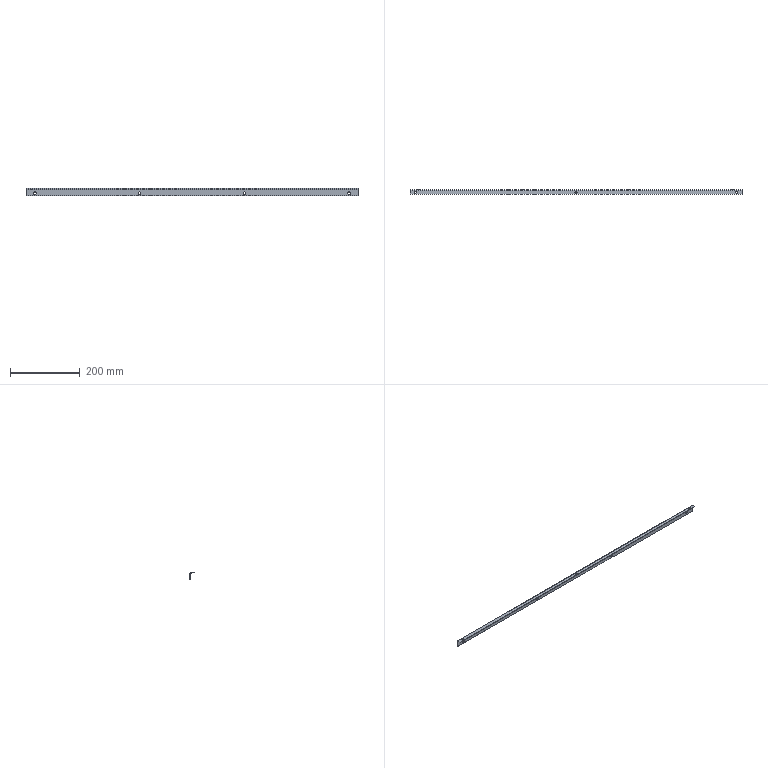Part | NX | features solid 2 | 1 solid | 24 faces | box 950 x 12.085 x 21.546 mm | volume 42798 mm3 | cylinder 16 | plane 8 | commonest cylinder face diameters 8.1 x8 6 x7 3 x1
STEP:
#1=CARTESIAN_POINT('',(626.,-1461.985,109.849));
#2=VERTEX_POINT('',#1);
#3=CARTESIAN_POINT('',(626.,-1462.116,108.354));
#4=VERTEX_POINT('',#3);
#5=CARTESIAN_POINT('',(626.,-1379.29,1055.059));
#6=DIRECTION('',(0.,-0.08716,-0.9962));
#7=VECTOR('',#6,1000.);
#8=LINE('',#5,#7);
#9=EDGE_CURVE('',#2,#4,#8,.T.);
#10=ORIENTED_EDGE('',*,*,#9,.F.);
#11=CARTESIAN_POINT('',(626.,-1467.962,110.372));
#12=VERTEX_POINT('',#11);
#13=CARTESIAN_POINT('',(626.,-1464.973,110.11));
#14=DIRECTION('',(0.,0.08716,0.9962));
#15=DIRECTION('',(0.,0.9962,-0.08716));
#16=AXIS2_PLACEMENT_3D('',#13,#14,#15);
#17=CIRCLE('',#16,3.);
#18=EDGE_CURVE('',#2,#12,#17,.T.);
#19=ORIENTED_EDGE('',*,*,#18,.T.);
#20=CARTESIAN_POINT('',(626.,-1468.093,108.877));
#21=VERTEX_POINT('',#20);
#22=CARTESIAN_POINT('',(626.,-1385.267,1055.582));
#23=DIRECTION('',(0.,-0.08716,-0.9962));
#24=VECTOR('',#23,1000.);
#25=LINE('',#22,#24);
#26=EDGE_CURVE('',#21,#12,#25,.F.);
#27=ORIENTED_EDGE('',*,*,#26,.F.);
#28=CARTESIAN_POINT('',(626.,-1465.104,108.616));
#29=DIRECTION('',(0.,-0.08716,-0.9962));
#30=DIRECTION('',(-1.,0.,0.));
#31=AXIS2_PLACEMENT_3D('',#28,#29,#30);
#32=CIRCLE('',#31,3.);
#33=EDGE_CURVE('',#21,#4,#32,.T.);
#34=ORIENTED_EDGE('',*,*,#33,.T.);
#35=EDGE_LOOP('',(#10,#19,#27,#34));
#36=FACE_BOUND('',#35,.T.);
#37=CARTESIAN_POINT('',(626.,-1382.278,1055.321));
#38=DIRECTION('',(0.,-0.08716,-0.9962));
#39=DIRECTION('',(0.,-0.9962,0.08716));
#40=AXIS2_PLACEMENT_3D('',#37,#38,#39);
#41=CYLINDRICAL_SURFACE('',#40,3.);
#42=ADVANCED_FACE('',(#36),#41,.F.);
#43=CARTESIAN_POINT('',(-294.,-1461.985,109.849));
#44=VERTEX_POINT('',#43);
#45=CARTESIAN_POINT('',(-294.,-1462.116,108.354));
#46=VERTEX_POINT('',#45);
#47=CARTESIAN_POINT('',(-294.,-1379.29,1055.059));
#48=DIRECTION('',(0.,-0.08716,-0.9962));
#49=VECTOR('',#48,1000.);
#50=LINE('',#47,#49);
#51=EDGE_CURVE('',#44,#46,#50,.T.);
#52=ORIENTED_EDGE('',*,*,#51,.F.);
#53=CARTESIAN_POINT('',(-294.,-1467.962,110.372));
#54=VERTEX_POINT('',#53);
#55=CARTESIAN_POINT('',(-294.,-1464.973,110.11));
#56=DIRECTION('',(0.,0.08716,0.9962));
#57=DIRECTION('',(0.,0.9962,-0.08716));
#58=AXIS2_PLACEMENT_3D('',#55,#56,#57);
#59=CIRCLE('',#58,3.);
#60=EDGE_CURVE('',#44,#54,#59,.T.);
#61=ORIENTED_EDGE('',*,*,#60,.T.);
#62=CARTESIAN_POINT('',(-294.,-1468.093,108.877));
#63=VERTEX_POINT('',#62);
#64=CARTESIAN_POINT('',(-294.,-1385.267,1055.582));
#65=DIRECTION('',(0.,-0.08716,-0.9962));
#66=VECTOR('',#65,1000.);
#67=LINE('',#64,#66);
#68=EDGE_CURVE('',#63,#54,#67,.F.);
#69=ORIENTED_EDGE('',*,*,#68,.F.);
#70=CARTESIAN_POINT('',(-294.,-1465.104,108.616));
#71=DIRECTION('',(0.,-0.08716,-0.9962));
#72=DIRECTION('',(-1.,0.,0.));
#73=AXIS2_PLACEMENT_3D('',#70,#71,#72);
#74=CIRCLE('',#73,3.);
#75=EDGE_CURVE('',#63,#46,#74,.T.);
#76=ORIENTED_EDGE('',*,*,#75,.T.);
#77=EDGE_LOOP('',(#52,#61,#69,#76));
#78=FACE_BOUND('',#77,.T.);
#79=CARTESIAN_POINT('',(-294.,-1382.278,1055.321));
#80=DIRECTION('',(0.,-0.08716,-0.9962));
#81=DIRECTION('',(0.,-0.9962,0.08716));
#82=AXIS2_PLACEMENT_3D('',#79,#80,#81);
#83=CYLINDRICAL_SURFACE('',#82,3.);
#84=ADVANCED_FACE('',(#78),#83,.F.);
#85=CARTESIAN_POINT('',(166.,-1461.985,109.849));
#86=VERTEX_POINT('',#85);
#87=CARTESIAN_POINT('',(166.,-1462.116,108.354));
#88=VERTEX_POINT('',#87);
#89=CARTESIAN_POINT('',(166.,-1379.29,1055.059));
#90=DIRECTION('',(0.,-0.08716,-0.9962));
#91=VECTOR('',#90,1000.);
#92=LINE('',#89,#91);
#93=EDGE_CURVE('',#86,#88,#92,.T.);
#94=ORIENTED_EDGE('',*,*,#93,.F.);
#95=CARTESIAN_POINT('',(166.,-1467.962,110.372));
#96=VERTEX_POINT('',#95);
#97=CARTESIAN_POINT('',(166.,-1464.973,110.11));
#98=DIRECTION('',(0.,0.08716,0.9962));
#99=DIRECTION('',(0.,0.9962,-0.08716));
#100=AXIS2_PLACEMENT_3D('',#97,#98,#99);
#101=CIRCLE('',#100,3.);
#102=EDGE_CURVE('',#86,#96,#101,.T.);
#103=ORIENTED_EDGE('',*,*,#102,.T.);
#104=CARTESIAN_POINT('',(166.,-1468.093,108.877));
#105=VERTEX_POINT('',#104);
#106=CARTESIAN_POINT('',(166.,-1385.267,1055.582));
#107=DIRECTION('',(0.,-0.08716,-0.9962));
#108=VECTOR('',#107,1000.);
#109=LINE('',#106,#108);
#110=EDGE_CURVE('',#105,#96,#109,.F.);
#111=ORIENTED_EDGE('',*,*,#110,.F.);
#112=CARTESIAN_POINT('',(166.,-1465.104,108.616));
#113=DIRECTION('',(0.,-0.08716,-0.9962));
#114=DIRECTION('',(-1.,0.,0.));
#115=AXIS2_PLACEMENT_3D('',#112,#113,#114);
#116=CIRCLE('',#115,3.);
#117=EDGE_CURVE('',#105,#88,#116,.T.);
#118=ORIENTED_EDGE('',*,*,#117,.T.);
#119=EDGE_LOOP('',(#94,#103,#111,#118));
#120=FACE_BOUND('',#119,.T.);
#121=CARTESIAN_POINT('',(166.,-1382.278,1055.321));
#122=DIRECTION('',(0.,-0.08716,-0.9962));
#123=DIRECTION('',(0.,-0.9962,0.08716));
#124=AXIS2_PLACEMENT_3D('',#121,#122,#123);
#125=CYLINDRICAL_SURFACE('',#124,3.);
#126=ADVANCED_FACE('',(#120),#125,.F.);
#127=CARTESIAN_POINT('',(-284.,-1459.5,91.95));
#128=VERTEX_POINT('',#127);
#129=CARTESIAN_POINT('',(-284.,-1458.,91.95));
#130=VERTEX_POINT('',#129);
#131=CARTESIAN_POINT('',(-284.,-509.179,91.95));
#132=DIRECTION('',(0.,-1.,0.));
#133=VECTOR('',#132,1000.);
#134=LINE('',#131,#133);
#135=EDGE_CURVE('',#128,#130,#134,.F.);
#136=ORIENTED_EDGE('',*,*,#135,.T.);
#137=CARTESIAN_POINT('',(-284.,-1458.,100.05));
#138=VERTEX_POINT('',#137);
#139=CARTESIAN_POINT('',(-284.,-1458.,96.));
#140=DIRECTION('',(0.,-1.,0.));
#141=DIRECTION('',(0.,0.,-1.));
#142=AXIS2_PLACEMENT_3D('',#139,#140,#141);
#143=CIRCLE('',#142,4.05);
#144=EDGE_CURVE('',#138,#130,#143,.T.);
#145=ORIENTED_EDGE('',*,*,#144,.F.);
#146=CARTESIAN_POINT('',(-284.,-1459.5,100.05));
#147=VERTEX_POINT('',#146);
#148=CARTESIAN_POINT('',(-284.,-509.179,100.05));
#149=DIRECTION('',(0.,-1.,0.));
#150=VECTOR('',#149,1000.);
#151=LINE('',#148,#150);
#152=EDGE_CURVE('',#138,#147,#151,.T.);
#153=ORIENTED_EDGE('',*,*,#152,.T.);
#154=CARTESIAN_POINT('',(-284.,-1459.5,96.));
#155=DIRECTION('',(0.,1.,0.));
#156=DIRECTION('',(1.,0.,0.));
#157=AXIS2_PLACEMENT_3D('',#154,#155,#156);
#158=CIRCLE('',#157,4.05);
#159=EDGE_CURVE('',#128,#147,#158,.T.);
#160=ORIENTED_EDGE('',*,*,#159,.F.);
#161=EDGE_LOOP('',(#136,#145,#153,#160));
#162=FACE_BOUND('',#161,.T.);
#163=CARTESIAN_POINT('',(-284.,-509.179,96.));
#164=DIRECTION('',(0.,-1.,0.));
#165=DIRECTION('',(0.,0.,1.));
#166=AXIS2_PLACEMENT_3D('',#163,#164,#165);
#167=CYLINDRICAL_SURFACE('',#166,4.05);
#168=ADVANCED_FACE('',(#162),#167,.F.);
#169=CARTESIAN_POINT('',(616.,-1459.5,91.95));
#170=VERTEX_POINT('',#169);
#171=CARTESIAN_POINT('',(616.,-1458.,91.95));
#172=VERTEX_POINT('',#171);
#173=CARTESIAN_POINT('',(616.,-509.179,91.95));
#174=DIRECTION('',(0.,-1.,0.));
#175=VECTOR('',#174,1000.);
#176=LINE('',#173,#175);
#177=EDGE_CURVE('',#170,#172,#176,.F.);
#178=ORIENTED_EDGE('',*,*,#177,.T.);
#179=CARTESIAN_POINT('',(616.,-1458.,100.05));
#180=VERTEX_POINT('',#179);
#181=CARTESIAN_POINT('',(616.,-1458.,96.));
#182=DIRECTION('',(0.,-1.,0.));
#183=DIRECTION('',(0.,0.,-1.));
#184=AXIS2_PLACEMENT_3D('',#181,#182,#183);
#185=CIRCLE('',#184,4.05);
#186=EDGE_CURVE('',#180,#172,#185,.T.);
#187=ORIENTED_EDGE('',*,*,#186,.F.);
#188=CARTESIAN_POINT('',(616.,-1459.5,100.05));
#189=VERTEX_POINT('',#188);
#190=CARTESIAN_POINT('',(616.,-509.179,100.05));
#191=DIRECTION('',(0.,-1.,0.));
#192=VECTOR('',#191,1000.);
#193=LINE('',#190,#192);
#194=EDGE_CURVE('',#180,#189,#193,.T.);
#195=ORIENTED_EDGE('',*,*,#194,.T.);
#196=CARTESIAN_POINT('',(616.,-1459.5,96.));
#197=DIRECTION('',(0.,1.,0.));
#198=DIRECTION('',(1.,0.,0.));
#199=AXIS2_PLACEMENT_3D('',#196,#197,#198);
#200=CIRCLE('',#199,4.05);
#201=EDGE_CURVE('',#170,#189,#200,.T.);
#202=ORIENTED_EDGE('',*,*,#201,.F.);
#203=EDGE_LOOP('',(#178,#187,#195,#202));
#204=FACE_BOUND('',#203,.T.);
#205=CARTESIAN_POINT('',(616.,-509.179,96.));
#206=DIRECTION('',(0.,-1.,0.));
#207=DIRECTION('',(0.,0.,1.));
#208=AXIS2_PLACEMENT_3D('',#205,#206,#207);
#209=CYLINDRICAL_SURFACE('',#208,4.05);
#210=ADVANCED_FACE('',(#204),#209,.F.);
#211=CARTESIAN_POINT('',(316.,-1458.,91.95));
#212=VERTEX_POINT('',#211);
#213=CARTESIAN_POINT('',(316.,-1459.5,91.95));
#214=VERTEX_POINT('',#213);
#215=CARTESIAN_POINT('',(316.,-509.179,91.95));
#216=DIRECTION('',(0.,-1.,0.));
#217=VECTOR('',#216,1000.);
#218=LINE('',#215,#217);
#219=EDGE_CURVE('',#212,#214,#218,.T.);
#220=ORIENTED_EDGE('',*,*,#219,.F.);
#221=CARTESIAN_POINT('',(316.,-1458.,100.05));
#222=VERTEX_POINT('',#221);
#223=CARTESIAN_POINT('',(316.,-1458.,96.));
#224=DIRECTION('',(0.,-1.,0.));
#225=DIRECTION('',(0.,0.,-1.));
#226=AXIS2_PLACEMENT_3D('',#223,#224,#225);
#227=CIRCLE('',#226,4.05);
#228=EDGE_CURVE('',#222,#212,#227,.T.);
#229=ORIENTED_EDGE('',*,*,#228,.F.);
#230=CARTESIAN_POINT('',(316.,-1459.5,100.05));
#231=VERTEX_POINT('',#230);
#232=CARTESIAN_POINT('',(316.,-509.179,100.05));
#233=DIRECTION('',(0.,-1.,0.));
#234=VECTOR('',#233,1000.);
#235=LINE('',#232,#234);
#236=EDGE_CURVE('',#231,#222,#235,.F.);
#237=ORIENTED_EDGE('',*,*,#236,.F.);
#238=CARTESIAN_POINT('',(316.,-1459.5,96.));
#239=DIRECTION('',(0.,1.,0.));
#240=DIRECTION('',(1.,0.,0.));
#241=AXIS2_PLACEMENT_3D('',#238,#239,#240);
#242=CIRCLE('',#241,4.05);
#243=EDGE_CURVE('',#214,#231,#242,.T.);
#244=ORIENTED_EDGE('',*,*,#243,.F.);
#245=EDGE_LOOP('',(#220,#229,#237,#244));
#246=FACE_BOUND('',#245,.T.);
#247=CARTESIAN_POINT('',(316.,-509.179,96.));
#248=DIRECTION('',(0.,-1.,0.));
#249=DIRECTION('',(0.,0.,1.));
#250=AXIS2_PLACEMENT_3D('',#247,#248,#249);
#251=CYLINDRICAL_SURFACE('',#250,4.05);
#252=ADVANCED_FACE('',(#246),#251,.F.);
#253=CARTESIAN_POINT('',(16.,-1459.5,91.95));
#254=VERTEX_POINT('',#253);
#255=CARTESIAN_POINT('',(16.,-1458.,91.95));
#256=VERTEX_POINT('',#255);
#257=CARTESIAN_POINT('',(16.,-509.179,91.95));
#258=DIRECTION('',(0.,-1.,0.));
#259=VECTOR('',#258,1000.);
#260=LINE('',#257,#259);
#261=EDGE_CURVE('',#254,#256,#260,.F.);
#262=ORIENTED_EDGE('',*,*,#261,.T.);
#263=CARTESIAN_POINT('',(16.,-1458.,100.05));
#264=VERTEX_POINT('',#263);
#265=CARTESIAN_POINT('',(16.,-1458.,96.));
#266=DIRECTION('',(0.,-1.,0.));
#267=DIRECTION('',(0.,0.,-1.));
#268=AXIS2_PLACEMENT_3D('',#265,#266,#267);
#269=CIRCLE('',#268,4.05);
#270=EDGE_CURVE('',#264,#256,#269,.T.);
#271=ORIENTED_EDGE('',*,*,#270,.F.);
#272=CARTESIAN_POINT('',(16.,-1459.5,100.05));
#273=VERTEX_POINT('',#272);
#274=CARTESIAN_POINT('',(16.,-509.179,100.05));
#275=DIRECTION('',(0.,-1.,0.));
#276=VECTOR('',#275,1000.);
#277=LINE('',#274,#276);
#278=EDGE_CURVE('',#264,#273,#277,.T.);
#279=ORIENTED_EDGE('',*,*,#278,.T.);
#280=CARTESIAN_POINT('',(16.,-1459.5,96.));
#281=DIRECTION('',(0.,1.,0.));
#282=DIRECTION('',(1.,0.,0.));
#283=AXIS2_PLACEMENT_3D('',#280,#281,#282);
#284=CIRCLE('',#283,4.05);
#285=EDGE_CURVE('',#254,#273,#284,.T.);
#286=ORIENTED_EDGE('',*,*,#285,.F.);
#287=EDGE_LOOP('',(#262,#271,#279,#286));
#288=FACE_BOUND('',#287,.T.);
#289=CARTESIAN_POINT('',(16.,-509.179,96.));
#290=DIRECTION('',(0.,-1.,0.));
#291=DIRECTION('',(0.,0.,1.));
#292=AXIS2_PLACEMENT_3D('',#289,#290,#291);
#293=CYLINDRICAL_SURFACE('',#292,4.05);
#294=ADVANCED_FACE('',(#288),#293,.F.);
#295=CARTESIAN_POINT('',(-309.,-1460.869,108.245));
#296=VERTEX_POINT('',#295);
#297=CARTESIAN_POINT('',(-309.,-1459.5,106.751));
#298=VERTEX_POINT('',#297);
#299=CARTESIAN_POINT('',(-309.,-1461.,106.751));
#300=DIRECTION('',(-1.,0.,0.));
#301=DIRECTION('',(0.,-1.,0.));
#302=AXIS2_PLACEMENT_3D('',#299,#300,#301);
#303=CIRCLE('',#302,1.5);
#304=EDGE_CURVE('',#296,#298,#303,.T.);
#305=ORIENTED_EDGE('',*,*,#304,.T.);
#306=CARTESIAN_POINT('',(641.,-1459.5,106.751));
#307=VERTEX_POINT('',#306);
#308=CARTESIAN_POINT('',(641.,-1459.5,106.751));
#309=DIRECTION('',(-1.,0.,0.));
#310=VECTOR('',#309,1000.);
#311=LINE('',#308,#310);
#312=EDGE_CURVE('',#307,#298,#311,.T.);
#313=ORIENTED_EDGE('',*,*,#312,.F.);
#314=CARTESIAN_POINT('',(641.,-1460.869,108.245));
#315=VERTEX_POINT('',#314);
#316=CARTESIAN_POINT('',(641.,-1461.,106.751));
#317=DIRECTION('',(-1.,0.,0.));
#318=DIRECTION('',(0.,-1.,0.));
#319=AXIS2_PLACEMENT_3D('',#316,#317,#318);
#320=CIRCLE('',#319,1.5);
#321=EDGE_CURVE('',#315,#307,#320,.T.);
#322=ORIENTED_EDGE('',*,*,#321,.F.);
#323=CARTESIAN_POINT('',(641.,-1460.869,108.245));
#324=DIRECTION('',(-1.,0.,0.));
#325=VECTOR('',#324,1000.);
#326=LINE('',#323,#325);
#327=EDGE_CURVE('',#315,#296,#326,.T.);
#328=ORIENTED_EDGE('',*,*,#327,.T.);
#329=EDGE_LOOP('',(#305,#313,#322,#328));
#330=FACE_BOUND('',#329,.T.);
#331=CARTESIAN_POINT('',(641.,-1461.,106.751));
#332=DIRECTION('',(-1.,0.,0.));
#333=DIRECTION('',(0.,-1.,0.));
#334=AXIS2_PLACEMENT_3D('',#331,#332,#333);
#335=CYLINDRICAL_SURFACE('',#334,1.5);
#336=ADVANCED_FACE('',(#330),#335,.F.);
#337=ORIENTED_EDGE('',*,*,#117,.F.);
#338=CARTESIAN_POINT('',(166.,-1465.104,108.616));
#339=DIRECTION('',(0.,-0.08716,-0.9962));
#340=DIRECTION('',(-1.,0.,0.));
#341=AXIS2_PLACEMENT_3D('',#338,#339,#340);
#342=CIRCLE('',#341,3.);
#343=EDGE_CURVE('',#88,#105,#342,.T.);
#344=ORIENTED_EDGE('',*,*,#343,.F.);
#345=EDGE_LOOP('',(#337,#344));
#346=FACE_BOUND('',#345,.T.);
#347=ORIENTED_EDGE('',*,*,#75,.F.);
#348=CARTESIAN_POINT('',(-294.,-1465.104,108.616));
#349=DIRECTION('',(0.,-0.08716,-0.9962));
#350=DIRECTION('',(-1.,0.,0.));
#351=AXIS2_PLACEMENT_3D('',#348,#349,#350);
#352=CIRCLE('',#351,3.);
#353=EDGE_CURVE('',#46,#63,#352,.T.);
#354=ORIENTED_EDGE('',*,*,#353,.F.);
#355=EDGE_LOOP('',(#347,#354));
#356=FACE_BOUND('',#355,.T.);
#357=ORIENTED_EDGE('',*,*,#33,.F.);
#358=CARTESIAN_POINT('',(626.,-1465.104,108.616));
#359=DIRECTION('',(0.,-0.08716,-0.9962));
#360=DIRECTION('',(-1.,0.,0.));
#361=AXIS2_PLACEMENT_3D('',#358,#359,#360);
#362=CIRCLE('',#361,3.);
#363=EDGE_CURVE('',#4,#21,#362,.T.);
#364=ORIENTED_EDGE('',*,*,#363,.F.);
#365=EDGE_LOOP('',(#357,#364));
#366=FACE_BOUND('',#365,.T.);
#367=CARTESIAN_POINT('',(-309.,-1470.085,109.052));
#368=VERTEX_POINT('',#367);
#369=CARTESIAN_POINT('',(-309.,-1470.085,109.052));
#370=DIRECTION('',(0.,0.9962,-0.08716));
#371=VECTOR('',#370,1000.);
#372=LINE('',#369,#371);
#373=EDGE_CURVE('',#368,#296,#372,.T.);
#374=ORIENTED_EDGE('',*,*,#373,.T.);
#375=ORIENTED_EDGE('',*,*,#327,.F.);
#376=CARTESIAN_POINT('',(641.,-1470.085,109.052));
#377=VERTEX_POINT('',#376);
#378=CARTESIAN_POINT('',(641.,-1470.085,109.052));
#379=DIRECTION('',(0.,0.9962,-0.08716));
#380=VECTOR('',#379,1000.);
#381=LINE('',#378,#380);
#382=EDGE_CURVE('',#377,#315,#381,.T.);
#383=ORIENTED_EDGE('',*,*,#382,.F.);
#384=CARTESIAN_POINT('',(641.,-1470.085,109.052));
#385=DIRECTION('',(-1.,0.,0.));
#386=VECTOR('',#385,1000.);
#387=LINE('',#384,#386);
#388=EDGE_CURVE('',#377,#368,#387,.T.);
#389=ORIENTED_EDGE('',*,*,#388,.T.);
#390=EDGE_LOOP('',(#374,#375,#383,#389));
#391=FACE_BOUND('',#390,.T.);
#392=CARTESIAN_POINT('',(641.,-1470.085,109.052));
#393=DIRECTION('',(0.,0.08716,0.9962));
#394=DIRECTION('',(1.,0.,0.));
#395=AXIS2_PLACEMENT_3D('',#392,#393,#394);
#396=PLANE('',#395);
#397=ADVANCED_FACE('',(#346,#356,#366,#391),#396,.F.);
#398=CARTESIAN_POINT('',(-309.,-1460.739,109.74));
#399=VERTEX_POINT('',#398);
#400=CARTESIAN_POINT('',(-309.,-1458.,106.751));
#401=VERTEX_POINT('',#400);
#402=CARTESIAN_POINT('',(-309.,-1461.,106.751));
#403=DIRECTION('',(-1.,0.,0.));
#404=DIRECTION('',(0.,1.,0.));
#405=AXIS2_PLACEMENT_3D('',#402,#403,#404);
#406=CIRCLE('',#405,3.);
#407=EDGE_CURVE('',#399,#401,#406,.T.);
#408=ORIENTED_EDGE('',*,*,#407,.F.);
#409=CARTESIAN_POINT('',(641.,-1460.739,109.74));
#410=VERTEX_POINT('',#409);
#411=CARTESIAN_POINT('',(641.,-1460.739,109.74));
#412=DIRECTION('',(-1.,0.,0.));
#413=VECTOR('',#412,1000.);
#414=LINE('',#411,#413);
#415=EDGE_CURVE('',#410,#399,#414,.T.);
#416=ORIENTED_EDGE('',*,*,#415,.F.);
#417=CARTESIAN_POINT('',(641.,-1458.,106.751));
#418=VERTEX_POINT('',#417);
#419=CARTESIAN_POINT('',(641.,-1461.,106.751));
#420=DIRECTION('',(-1.,0.,0.));
#421=DIRECTION('',(0.,1.,0.));
#422=AXIS2_PLACEMENT_3D('',#419,#420,#421);
#423=CIRCLE('',#422,3.);
#424=EDGE_CURVE('',#410,#418,#423,.T.);
#425=ORIENTED_EDGE('',*,*,#424,.T.);
#426=CARTESIAN_POINT('',(641.,-1458.,106.751));
#427=DIRECTION('',(-1.,0.,0.));
#428=VECTOR('',#427,1000.);
#429=LINE('',#426,#428);
#430=EDGE_CURVE('',#418,#401,#429,.T.);
#431=ORIENTED_EDGE('',*,*,#430,.T.);
#432=EDGE_LOOP('',(#408,#416,#425,#431));
#433=FACE_BOUND('',#432,.T.);
#434=CARTESIAN_POINT('',(641.,-1461.,106.751));
#435=DIRECTION('',(-1.,0.,0.));
#436=DIRECTION('',(0.,-1.,0.));
#437=AXIS2_PLACEMENT_3D('',#434,#435,#436);
#438=CYLINDRICAL_SURFACE('',#437,3.);
#439=ADVANCED_FACE('',(#433),#438,.T.);
#440=CARTESIAN_POINT('',(166.,-1464.973,110.11));
#441=DIRECTION('',(0.,0.08716,0.9962));
#442=DIRECTION('',(0.,0.9962,-0.08716));
#443=AXIS2_PLACEMENT_3D('',#440,#441,#442);
#444=CIRCLE('',#443,3.);
#445=EDGE_CURVE('',#96,#86,#444,.T.);
#446=ORIENTED_EDGE('',*,*,#445,.F.);
#447=ORIENTED_EDGE('',*,*,#102,.F.);
#448=EDGE_LOOP('',(#446,#447));
#449=FACE_BOUND('',#448,.T.);
#450=CARTESIAN_POINT('',(-294.,-1464.973,110.11));
#451=DIRECTION('',(0.,0.08716,0.9962));
#452=DIRECTION('',(0.,0.9962,-0.08716));
#453=AXIS2_PLACEMENT_3D('',#450,#451,#452);
#454=CIRCLE('',#453,3.);
#455=EDGE_CURVE('',#54,#44,#454,.T.);
#456=ORIENTED_EDGE('',*,*,#455,.F.);
#457=ORIENTED_EDGE('',*,*,#60,.F.);
#458=EDGE_LOOP('',(#456,#457));
#459=FACE_BOUND('',#458,.T.);
#460=CARTESIAN_POINT('',(626.,-1464.973,110.11));
#461=DIRECTION('',(0.,0.08716,0.9962));
#462=DIRECTION('',(0.,0.9962,-0.08716));
#463=AXIS2_PLACEMENT_3D('',#460,#461,#462);
#464=CIRCLE('',#463,3.);
#465=EDGE_CURVE('',#12,#2,#464,.T.);
#466=ORIENTED_EDGE('',*,*,#465,.F.);
#467=ORIENTED_EDGE('',*,*,#18,.F.);
#468=EDGE_LOOP('',(#466,#467));
#469=FACE_BOUND('',#468,.T.);
#470=CARTESIAN_POINT('',(-309.,-1469.954,110.546));
#471=VERTEX_POINT('',#470);
#472=CARTESIAN_POINT('',(-309.,-1469.954,110.546));
#473=DIRECTION('',(0.,0.9962,-0.08716));
#474=VECTOR('',#473,1000.);
#475=LINE('',#472,#474);
#476=EDGE_CURVE('',#471,#399,#475,.T.);
#477=ORIENTED_EDGE('',*,*,#476,.F.);
#478=CARTESIAN_POINT('',(641.,-1469.954,110.546));
#479=VERTEX_POINT('',#478);
#480=CARTESIAN_POINT('',(641.,-1469.954,110.546));
#481=DIRECTION('',(-1.,0.,0.));
#482=VECTOR('',#481,1000.);
#483=LINE('',#480,#482);
#484=EDGE_CURVE('',#479,#471,#483,.T.);
#485=ORIENTED_EDGE('',*,*,#484,.F.);
#486=CARTESIAN_POINT('',(641.,-1469.954,110.546));
#487=DIRECTION('',(0.,0.9962,-0.08716));
#488=VECTOR('',#487,1000.);
#489=LINE('',#486,#488);
#490=EDGE_CURVE('',#479,#410,#489,.T.);
#491=ORIENTED_EDGE('',*,*,#490,.T.);
#492=ORIENTED_EDGE('',*,*,#415,.T.);
#493=EDGE_LOOP('',(#477,#485,#491,#492));
#494=FACE_BOUND('',#493,.T.);
#495=CARTESIAN_POINT('',(641.,-1469.954,110.546));
#496=DIRECTION('',(0.,0.08716,0.9962));
#497=DIRECTION('',(1.,0.,0.));
#498=AXIS2_PLACEMENT_3D('',#495,#496,#497);
#499=PLANE('',#498);
#500=ADVANCED_FACE('',(#449,#459,#469,#494),#499,.T.);
#501=ORIENTED_EDGE('',*,*,#388,.F.);
#502=CARTESIAN_POINT('',(641.,-1469.954,110.546));
#503=DIRECTION('',(0.,0.08716,0.9962));
#504=VECTOR('',#503,1000.);
#505=LINE('',#502,#504);
#506=EDGE_CURVE('',#377,#479,#505,.T.);
#507=ORIENTED_EDGE('',*,*,#506,.T.);
#508=ORIENTED_EDGE('',*,*,#484,.T.);
#509=CARTESIAN_POINT('',(-309.,-1469.954,110.546));
#510=DIRECTION('',(0.,0.08716,0.9962));
#511=VECTOR('',#510,1000.);
#512=LINE('',#509,#511);
#513=EDGE_CURVE('',#368,#471,#512,.T.);
#514=ORIENTED_EDGE('',*,*,#513,.F.);
#515=EDGE_LOOP('',(#501,#507,#508,#514));
#516=FACE_BOUND('',#515,.T.);
#517=CARTESIAN_POINT('',(641.,-1469.954,110.546));
#518=DIRECTION('',(0.,0.9962,-0.08716));
#519=DIRECTION('',(-1.,0.,0.));
#520=AXIS2_PLACEMENT_3D('',#517,#518,#519);
#521=PLANE('',#520);
#522=ADVANCED_FACE('',(#516),#521,.F.);
#523=ORIENTED_EDGE('',*,*,#476,.T.);
#524=ORIENTED_EDGE('',*,*,#407,.T.);
#525=CARTESIAN_POINT('',(-309.,-1458.,89.));
#526=VERTEX_POINT('',#525);
#527=CARTESIAN_POINT('',(-309.,-1458.,109.5));
#528=DIRECTION('',(0.,0.,-1.));
#529=VECTOR('',#528,1000.);
#530=LINE('',#527,#529);
#531=EDGE_CURVE('',#401,#526,#530,.T.);
#532=ORIENTED_EDGE('',*,*,#531,.T.);
#533=CARTESIAN_POINT('',(-309.,-1459.5,89.));
#534=VERTEX_POINT('',#533);
#535=CARTESIAN_POINT('',(-309.,-1458.,89.));
#536=DIRECTION('',(0.,1.,0.));
#537=VECTOR('',#536,1000.);
#538=LINE('',#535,#537);
#539=EDGE_CURVE('',#534,#526,#538,.T.);
#540=ORIENTED_EDGE('',*,*,#539,.F.);
#541=CARTESIAN_POINT('',(-309.,-1459.5,109.5));
#542=DIRECTION('',(0.,0.,-1.));
#543=VECTOR('',#542,1000.);
#544=LINE('',#541,#543);
#545=EDGE_CURVE('',#298,#534,#544,.T.);
#546=ORIENTED_EDGE('',*,*,#545,.F.);
#547=ORIENTED_EDGE('',*,*,#304,.F.);
#548=ORIENTED_EDGE('',*,*,#373,.F.);
#549=ORIENTED_EDGE('',*,*,#513,.T.);
#550=EDGE_LOOP('',(#523,#524,#532,#540,#546,#547,#548,#549));
#551=FACE_BOUND('',#550,.T.);
#552=CARTESIAN_POINT('',(-309.,-1469.954,110.546));
#553=DIRECTION('',(1.,0.,0.));
#554=DIRECTION('',(0.,-1.,0.));
#555=AXIS2_PLACEMENT_3D('',#552,#553,#554);
#556=PLANE('',#555);
#557=ADVANCED_FACE('',(#551),#556,.F.);
#558=CARTESIAN_POINT('',(641.,-1459.5,89.));
#559=VERTEX_POINT('',#558);
#560=CARTESIAN_POINT('',(641.,-1458.,89.));
#561=VERTEX_POINT('',#560);
#562=CARTESIAN_POINT('',(641.,-1458.,89.));
#563=DIRECTION('',(0.,1.,0.));
#564=VECTOR('',#563,1000.);
#565=LINE('',#562,#564);
#566=EDGE_CURVE('',#559,#561,#565,.T.);
#567=ORIENTED_EDGE('',*,*,#566,.F.);
#568=CARTESIAN_POINT('',(641.,-1459.5,89.));
#569=DIRECTION('',(-1.,0.,0.));
#570=VECTOR('',#569,1000.);
#571=LINE('',#568,#570);
#572=EDGE_CURVE('',#559,#534,#571,.T.);
#573=ORIENTED_EDGE('',*,*,#572,.T.);
#574=ORIENTED_EDGE('',*,*,#539,.T.);
#575=CARTESIAN_POINT('',(641.,-1458.,89.));
#576=DIRECTION('',(-1.,0.,0.));
#577=VECTOR('',#576,1000.);
#578=LINE('',#575,#577);
#579=EDGE_CURVE('',#561,#526,#578,.T.);
#580=ORIENTED_EDGE('',*,*,#579,.F.);
#581=EDGE_LOOP('',(#567,#573,#574,#580));
#582=FACE_BOUND('',#581,.T.);
#583=CARTESIAN_POINT('',(641.,-1458.,89.));
#584=DIRECTION('',(0.,0.,-1.));
#585=DIRECTION('',(0.,-1.,0.));
#586=AXIS2_PLACEMENT_3D('',#583,#584,#585);
#587=PLANE('',#586);
#588=ADVANCED_FACE('',(#582),#587,.T.);
#589=CARTESIAN_POINT('',(641.,-1458.,109.5));
#590=DIRECTION('',(0.,0.,-1.));
#591=VECTOR('',#590,1000.);
#592=LINE('',#589,#591);
#593=EDGE_CURVE('',#418,#561,#592,.T.);
#594=ORIENTED_EDGE('',*,*,#593,.F.);
#595=ORIENTED_EDGE('',*,*,#424,.F.);
#596=ORIENTED_EDGE('',*,*,#490,.F.);
#597=ORIENTED_EDGE('',*,*,#506,.F.);
#598=ORIENTED_EDGE('',*,*,#382,.T.);
#599=ORIENTED_EDGE('',*,*,#321,.T.);
#600=CARTESIAN_POINT('',(641.,-1459.5,109.5));
#601=DIRECTION('',(0.,0.,-1.));
#602=VECTOR('',#601,1000.);
#603=LINE('',#600,#602);
#604=EDGE_CURVE('',#307,#559,#603,.T.);
#605=ORIENTED_EDGE('',*,*,#604,.T.);
#606=ORIENTED_EDGE('',*,*,#566,.T.);
#607=EDGE_LOOP('',(#594,#595,#596,#597,#598,#599,#605,#606));
#608=FACE_BOUND('',#607,.T.);
#609=CARTESIAN_POINT('',(641.,-1458.,109.5));
#610=DIRECTION('',(1.,0.,0.));
#611=DIRECTION('',(0.,-1.,0.));
#612=AXIS2_PLACEMENT_3D('',#609,#610,#611);
#613=PLANE('',#612);
#614=ADVANCED_FACE('',(#608),#613,.T.);
#615=CARTESIAN_POINT('',(-284.,-1459.5,96.));
#616=DIRECTION('',(0.,1.,0.));
#617=DIRECTION('',(1.,0.,0.));
#618=AXIS2_PLACEMENT_3D('',#615,#616,#617);
#619=CIRCLE('',#618,4.05);
#620=EDGE_CURVE('',#147,#128,#619,.T.);
#621=ORIENTED_EDGE('',*,*,#620,.T.);
#622=ORIENTED_EDGE('',*,*,#159,.T.);
#623=EDGE_LOOP('',(#621,#622));
#624=FACE_BOUND('',#623,.T.);
#625=CARTESIAN_POINT('',(316.,-1459.5,96.));
#626=DIRECTION('',(0.,1.,0.));
#627=DIRECTION('',(1.,0.,0.));
#628=AXIS2_PLACEMENT_3D('',#625,#626,#627);
#629=CIRCLE('',#628,4.05);
#630=EDGE_CURVE('',#231,#214,#629,.T.);
#631=ORIENTED_EDGE('',*,*,#630,.T.);
#632=ORIENTED_EDGE('',*,*,#243,.T.);
#633=EDGE_LOOP('',(#631,#632));
#634=FACE_BOUND('',#633,.T.);
#635=CARTESIAN_POINT('',(16.,-1459.5,96.));
#636=DIRECTION('',(0.,1.,0.));
#637=DIRECTION('',(1.,0.,0.));
#638=AXIS2_PLACEMENT_3D('',#635,#636,#637);
#639=CIRCLE('',#638,4.05);
#640=EDGE_CURVE('',#273,#254,#639,.T.);
#641=ORIENTED_EDGE('',*,*,#640,.T.);
#642=ORIENTED_EDGE('',*,*,#285,.T.);
#643=EDGE_LOOP('',(#641,#642));
#644=FACE_BOUND('',#643,.T.);
#645=CARTESIAN_POINT('',(616.,-1459.5,96.));
#646=DIRECTION('',(0.,1.,0.));
#647=DIRECTION('',(1.,0.,0.));
#648=AXIS2_PLACEMENT_3D('',#645,#646,#647);
#649=CIRCLE('',#648,4.05);
#650=EDGE_CURVE('',#189,#170,#649,.T.);
#651=ORIENTED_EDGE('',*,*,#650,.T.);
#652=ORIENTED_EDGE('',*,*,#201,.T.);
#653=EDGE_LOOP('',(#651,#652));
#654=FACE_BOUND('',#653,.T.);
#655=ORIENTED_EDGE('',*,*,#545,.T.);
#656=ORIENTED_EDGE('',*,*,#572,.F.);
#657=ORIENTED_EDGE('',*,*,#604,.F.);
#658=ORIENTED_EDGE('',*,*,#312,.T.);
#659=EDGE_LOOP('',(#655,#656,#657,#658));
#660=FACE_BOUND('',#659,.T.);
#661=CARTESIAN_POINT('',(641.,-1459.5,109.5));
#662=DIRECTION('',(0.,1.,0.));
#663=DIRECTION('',(0.,0.,-1.));
#664=AXIS2_PLACEMENT_3D('',#661,#662,#663);
#665=PLANE('',#664);
#666=ADVANCED_FACE('',(#624,#634,#644,#654,#660),#665,.F.);
#667=ORIENTED_EDGE('',*,*,#144,.T.);
#668=CARTESIAN_POINT('',(-284.,-1458.,96.));
#669=DIRECTION('',(0.,-1.,0.));
#670=DIRECTION('',(0.,0.,-1.));
#671=AXIS2_PLACEMENT_3D('',#668,#669,#670);
#672=CIRCLE('',#671,4.05);
#673=EDGE_CURVE('',#130,#138,#672,.T.);
#674=ORIENTED_EDGE('',*,*,#673,.T.);
#675=EDGE_LOOP('',(#667,#674));
#676=FACE_BOUND('',#675,.T.);
#677=ORIENTED_EDGE('',*,*,#228,.T.);
#678=CARTESIAN_POINT('',(316.,-1458.,96.));
#679=DIRECTION('',(0.,-1.,0.));
#680=DIRECTION('',(0.,0.,-1.));
#681=AXIS2_PLACEMENT_3D('',#678,#679,#680);
#682=CIRCLE('',#681,4.05);
#683=EDGE_CURVE('',#212,#222,#682,.T.);
#684=ORIENTED_EDGE('',*,*,#683,.T.);
#685=EDGE_LOOP('',(#677,#684));
#686=FACE_BOUND('',#685,.T.);
#687=ORIENTED_EDGE('',*,*,#270,.T.);
#688=CARTESIAN_POINT('',(16.,-1458.,96.));
#689=DIRECTION('',(0.,-1.,0.));
#690=DIRECTION('',(0.,0.,-1.));
#691=AXIS2_PLACEMENT_3D('',#688,#689,#690);
#692=CIRCLE('',#691,4.05);
#693=EDGE_CURVE('',#256,#264,#692,.T.);
#694=ORIENTED_EDGE('',*,*,#693,.T.);
#695=EDGE_LOOP('',(#687,#694));
#696=FACE_BOUND('',#695,.T.);
#697=ORIENTED_EDGE('',*,*,#186,.T.);
#698=CARTESIAN_POINT('',(616.,-1458.,96.));
#699=DIRECTION('',(0.,-1.,0.));
#700=DIRECTION('',(0.,0.,-1.));
#701=AXIS2_PLACEMENT_3D('',#698,#699,#700);
#702=CIRCLE('',#701,4.05);
#703=EDGE_CURVE('',#172,#180,#702,.T.);
#704=ORIENTED_EDGE('',*,*,#703,.T.);
#705=EDGE_LOOP('',(#697,#704));
#706=FACE_BOUND('',#705,.T.);
#707=ORIENTED_EDGE('',*,*,#531,.F.);
#708=ORIENTED_EDGE('',*,*,#430,.F.);
#709=ORIENTED_EDGE('',*,*,#593,.T.);
#710=ORIENTED_EDGE('',*,*,#579,.T.);
#711=EDGE_LOOP('',(#707,#708,#709,#710));
#712=FACE_BOUND('',#711,.T.);
#713=CARTESIAN_POINT('',(641.,-1458.,109.5));
#714=DIRECTION('',(0.,1.,0.));
#715=DIRECTION('',(0.,0.,-1.));
#716=AXIS2_PLACEMENT_3D('',#713,#714,#715);
#717=PLANE('',#716);
#718=ADVANCED_FACE('',(#676,#686,#696,#706,#712),#717,.T.);
#719=ORIENTED_EDGE('',*,*,#693,.F.);
#720=ORIENTED_EDGE('',*,*,#261,.F.);
#721=ORIENTED_EDGE('',*,*,#640,.F.);
#722=ORIENTED_EDGE('',*,*,#278,.F.);
#723=EDGE_LOOP('',(#719,#720,#721,#722));
#724=FACE_BOUND('',#723,.T.);
#725=CARTESIAN_POINT('',(16.,-509.179,96.));
#726=DIRECTION('',(0.,-1.,0.));
#727=DIRECTION('',(0.,0.,1.));
#728=AXIS2_PLACEMENT_3D('',#725,#726,#727);
#729=CYLINDRICAL_SURFACE('',#728,4.05);
#730=ADVANCED_FACE('',(#724),#729,.F.);
#731=ORIENTED_EDGE('',*,*,#683,.F.);
#732=ORIENTED_EDGE('',*,*,#219,.T.);
#733=ORIENTED_EDGE('',*,*,#630,.F.);
#734=ORIENTED_EDGE('',*,*,#236,.T.);
#735=EDGE_LOOP('',(#731,#732,#733,#734));
#736=FACE_BOUND('',#735,.T.);
#737=CARTESIAN_POINT('',(316.,-509.179,96.));
#738=DIRECTION('',(0.,-1.,0.));
#739=DIRECTION('',(0.,0.,1.));
#740=AXIS2_PLACEMENT_3D('',#737,#738,#739);
#741=CYLINDRICAL_SURFACE('',#740,4.05);
#742=ADVANCED_FACE('',(#736),#741,.F.);
#743=ORIENTED_EDGE('',*,*,#703,.F.);
#744=ORIENTED_EDGE('',*,*,#177,.F.);
#745=ORIENTED_EDGE('',*,*,#650,.F.);
#746=ORIENTED_EDGE('',*,*,#194,.F.);
#747=EDGE_LOOP('',(#743,#744,#745,#746));
#748=FACE_BOUND('',#747,.T.);
#749=CARTESIAN_POINT('',(616.,-509.179,96.));
#750=DIRECTION('',(0.,-1.,0.));
#751=DIRECTION('',(0.,0.,1.));
#752=AXIS2_PLACEMENT_3D('',#749,#750,#751);
#753=CYLINDRICAL_SURFACE('',#752,4.05);
#754=ADVANCED_FACE('',(#748),#753,.F.);
#755=ORIENTED_EDGE('',*,*,#673,.F.);
#756=ORIENTED_EDGE('',*,*,#135,.F.);
#757=ORIENTED_EDGE('',*,*,#620,.F.);
#758=ORIENTED_EDGE('',*,*,#152,.F.);
#759=EDGE_LOOP('',(#755,#756,#757,#758));
#760=FACE_BOUND('',#759,.T.);
#761=CARTESIAN_POINT('',(-284.,-509.179,96.));
#762=DIRECTION('',(0.,-1.,0.));
#763=DIRECTION('',(0.,0.,1.));
#764=AXIS2_PLACEMENT_3D('',#761,#762,#763);
#765=CYLINDRICAL_SURFACE('',#764,4.05);
#766=ADVANCED_FACE('',(#760),#765,.F.);
#767=ORIENTED_EDGE('',*,*,#445,.T.);
#768=ORIENTED_EDGE('',*,*,#93,.T.);
#769=ORIENTED_EDGE('',*,*,#343,.T.);
#770=ORIENTED_EDGE('',*,*,#110,.T.);
#771=EDGE_LOOP('',(#767,#768,#769,#770));
#772=FACE_BOUND('',#771,.T.);
#773=CARTESIAN_POINT('',(166.,-1382.278,1055.321));
#774=DIRECTION('',(0.,-0.08716,-0.9962));
#775=DIRECTION('',(0.,-0.9962,0.08716));
#776=AXIS2_PLACEMENT_3D('',#773,#774,#775);
#777=CYLINDRICAL_SURFACE('',#776,3.);
#778=ADVANCED_FACE('',(#772),#777,.F.);
#779=ORIENTED_EDGE('',*,*,#455,.T.);
#780=ORIENTED_EDGE('',*,*,#51,.T.);
#781=ORIENTED_EDGE('',*,*,#353,.T.);
#782=ORIENTED_EDGE('',*,*,#68,.T.);
#783=EDGE_LOOP('',(#779,#780,#781,#782));
#784=FACE_BOUND('',#783,.T.);
#785=CARTESIAN_POINT('',(-294.,-1382.278,1055.321));
#786=DIRECTION('',(0.,-0.08716,-0.9962));
#787=DIRECTION('',(0.,-0.9962,0.08716));
#788=AXIS2_PLACEMENT_3D('',#785,#786,#787);
#789=CYLINDRICAL_SURFACE('',#788,3.);
#790=ADVANCED_FACE('',(#784),#789,.F.);
#791=ORIENTED_EDGE('',*,*,#465,.T.);
#792=ORIENTED_EDGE('',*,*,#9,.T.);
#793=ORIENTED_EDGE('',*,*,#363,.T.);
#794=ORIENTED_EDGE('',*,*,#26,.T.);
#795=EDGE_LOOP('',(#791,#792,#793,#794));
#796=FACE_BOUND('',#795,.T.);
#797=CARTESIAN_POINT('',(626.,-1382.278,1055.321));
#798=DIRECTION('',(0.,-0.08716,-0.9962));
#799=DIRECTION('',(0.,-0.9962,0.08716));
#800=AXIS2_PLACEMENT_3D('',#797,#798,#799);
#801=CYLINDRICAL_SURFACE('',#800,3.);
#802=ADVANCED_FACE('',(#796),#801,.F.);
#803=CLOSED_SHELL('',(#42,#84,#126,#168,#210,#252,#294,#336,#397,#439,#500,#522,#557,#588,#614,#666,#718,#730,#742,#754,#766,#778,#790,#802));
#804=MANIFOLD_SOLID_BREP('',#803);
#805=(LENGTH_UNIT()NAMED_UNIT(*)SI_UNIT(.MILLI.,.METRE.));
#806=UNCERTAINTY_MEASURE_WITH_UNIT(LENGTH_MEASURE(0.00001),#805,'','');
#807=(NAMED_UNIT(*)PLANE_ANGLE_UNIT()SI_UNIT($,.RADIAN.));
#808=(NAMED_UNIT(*)SI_UNIT($,.STERADIAN.)SOLID_ANGLE_UNIT());
#809=(GEOMETRIC_REPRESENTATION_CONTEXT(3)GLOBAL_UNCERTAINTY_ASSIGNED_CONTEXT((#806))GLOBAL_UNIT_ASSIGNED_CONTEXT((#805,#807,#808))REPRESENTATION_CONTEXT('',''));
#810=ADVANCED_BREP_SHAPE_REPRESENTATION('',(#804),#809);